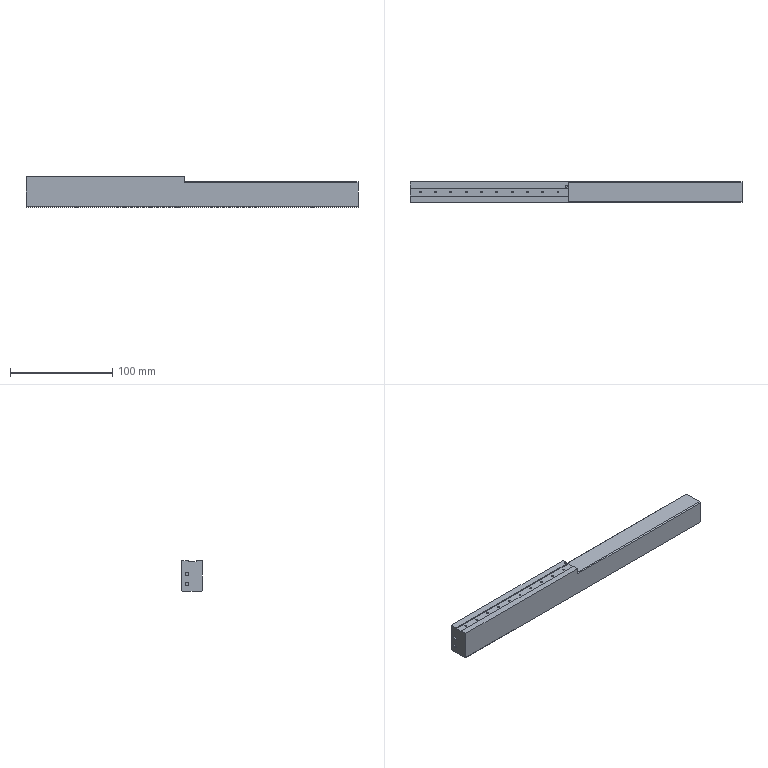CAM job | NX | 3-axis milling, drilling | part box 325 x 20 x 30 mm | stock box 333 x 28 x 31 mm
Tools:
number,name,description,diameter,corner_radius,flute_length,length,flutes
1,D63,Milling Tool-5 Parameters,63.0,0.0,50.0,75.0,2
10,D10,Milling Tool-5 Parameters,10.0,0.0,50.0,75.0,2
7,D6A45,Milling Tool-5 Parameters,6.0,0.0,3.0,3.0,2
13,M2,Milling Tool-5 Parameters,1.7,0.0,30.0,30.0,4
17,1.7ZT,Drilling Tool,1.7,0.0,35.0,50.0,2
11,D10JING,Milling Tool-5 Parameters,10.0,0.0,50.0,75.0,2
6,D6,Milling Tool-5 Parameters,6.0,0.0,50.0,75.0,2
Operations:
program,operation,operation_type,tool,method,geometry_group,spindle_rpm,surface_speed,feed_per_tooth,feed_cut,feed_plunge,cut_length_mm,path_length_mm,cut_time_min,machine_time_min
1-25-35-330毛胚,FLOOR_WALL,VolumeBased25DMillingOperation,D63,METHOD,A,6500.0,1286.0,0.0962,1250.0,100.0,408.0,462.0,0.3264,0.3318
1-25-35-330毛胚,ADAPTIVE_MILLING,CavityMilling,D10,METHOD,A,7000.0,219.0,0.2143,3000.0,1000.0,12681.597,17464.705,4.277,4.755
1-25-35-330毛胚,DRILLING_COPY_1,Operation,D6A45,METHOD,A,3000.0,56.0,0.0333,200.0,0.0,44.0,325.835,0.22,0.2482
1-25-35-330毛胚,DRILLING_COPY_1_COPY,Operation,1.7ZT,METHOD,A,2000.0,15.0,0.0375,120.0,0.0,170.618,579.071,1.422,1.463
1-25-35-330毛胚,DRILLING_COPY_1_COPY_COPY,Operation,M2,METHOD,A,200.0,1.0,0.125,80.0,0.0,143.0,523.835,1.788,1.826
1-25-35-330毛胚,ZLEVEL_PROFILE_COPY_COPY_1_COPY_COPY_COPY_1,ZLevelMilling,D10JING,METHOD,A,7000.0,219.0,0.0714,1000.0,100.0,1449.097,1569.265,1.449,1.461
1-25-35-330毛胚,FLOOR_WALL_1_COPY_1,VolumeBased25DMillingOperation,D10JING,METHOD,A,7000.0,87.0,0.0714,1000.0,100.0,1192.041,1293.245,1.192,1.204
1-25-35-330毛胚,ZLEVEL_PROFILE_COPY_COPY_1_COPY_COPY_COPY_1_COPY,ZLevelMilling,D6,METHOD,A,7000.0,219.0,0.0714,1000.0,100.0,653.627,1001.97,0.6536,0.6885
1-25-35-330毛胚,ZLEVEL_PROFILE_COPY_1_COPY_COPY_COPY_COPY_2_COPY,ZLevelMilling,D6A45,METHOD,A,7000.0,131.0,0.0714,1000.0,1000.0,660.688,940.562,0.6607,0.6887
1-25-35-330毛胚,ZLEVEL_PROFILE_COPY_1_COPY_COPY_COPY_COPY_2_COPY_COPY,ZLevelMilling,D6A45,METHOD,A,7000.0,131.0,0.0714,1000.0,1000.0,359.005,432.005,0.359,0.3663
1-25-35-330毛胚,DRILLING_COPY_1_COPY_1,Operation,D6A45,METHOD,A,3000.0,56.0,0.0333,200.0,0.0,45.1,328.786,0.2255,0.2539